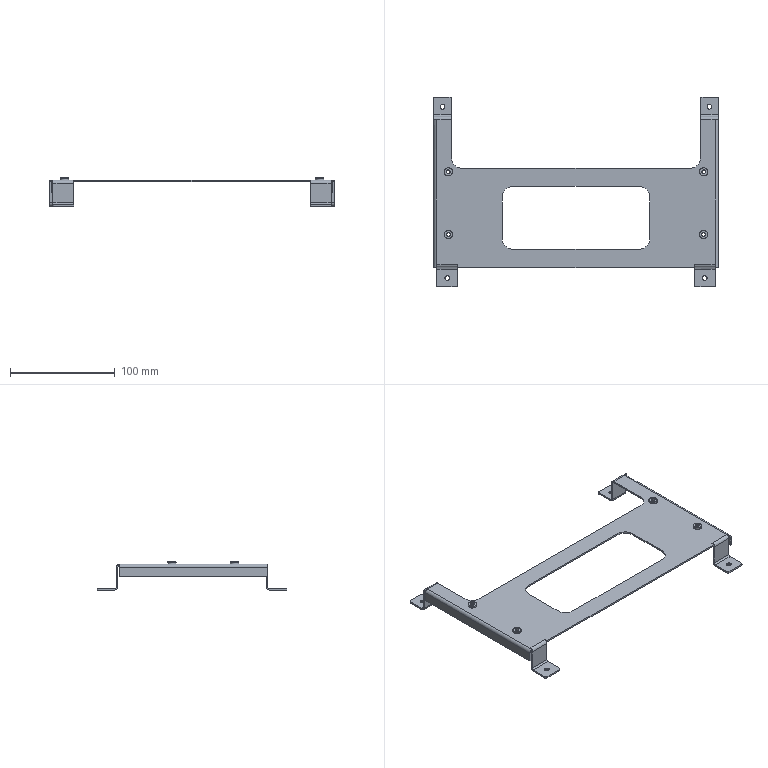Part | NX | features BREP 2 | 5 solids | 750 faces | box 272 x 181.457 x 26.9 mm | volume 37450 mm3 | plane 644 | cylinder 74 | cone 32 | commonest cylinder face diameters 3 x18 4.5 x16 6 x10 3.3 x8 5.38 x8 8 x8